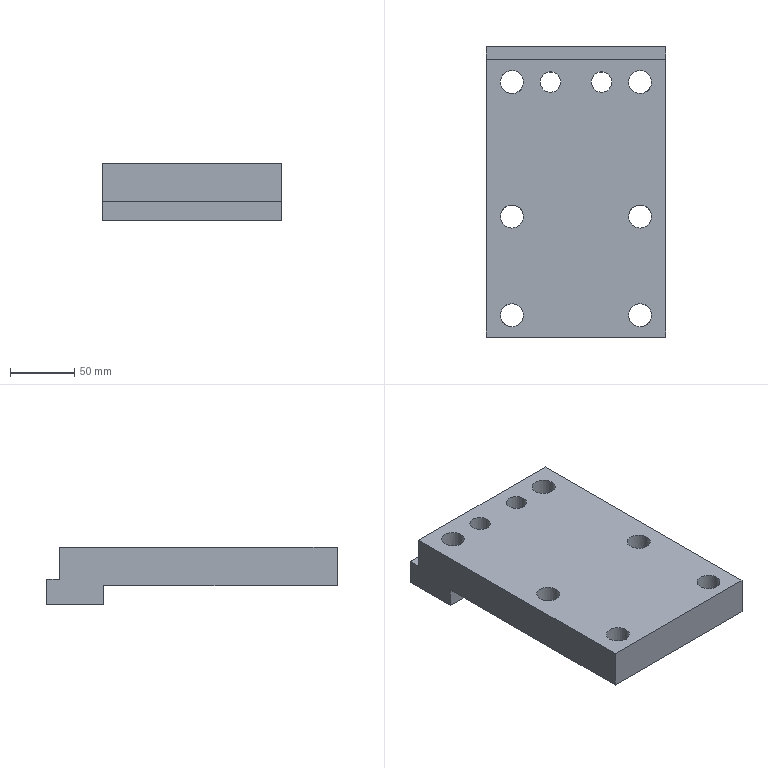Part | STEP file | solid 225 | 1 solid | 30 faces | box 140 x 226.5 x 45 mm | volume 911767 mm3 | plane 16 | cylinder 14 | commonest cylinder face diameters 18 x6 26 x6 16 x2